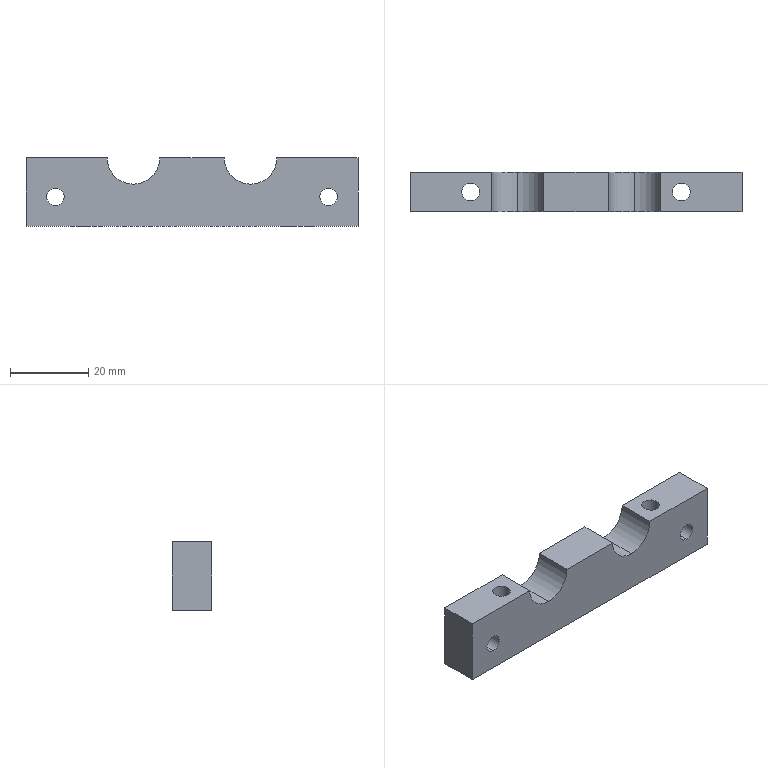Part | STEP file | Station two plug plate up | 1 solid | 32 faces | box 85 x 10 x 17.5 mm | volume 11964 mm3 | cylinder 20 | plane 12 | commonest cylinder face diameters 4.5 x8 8 x8 13.5 x4